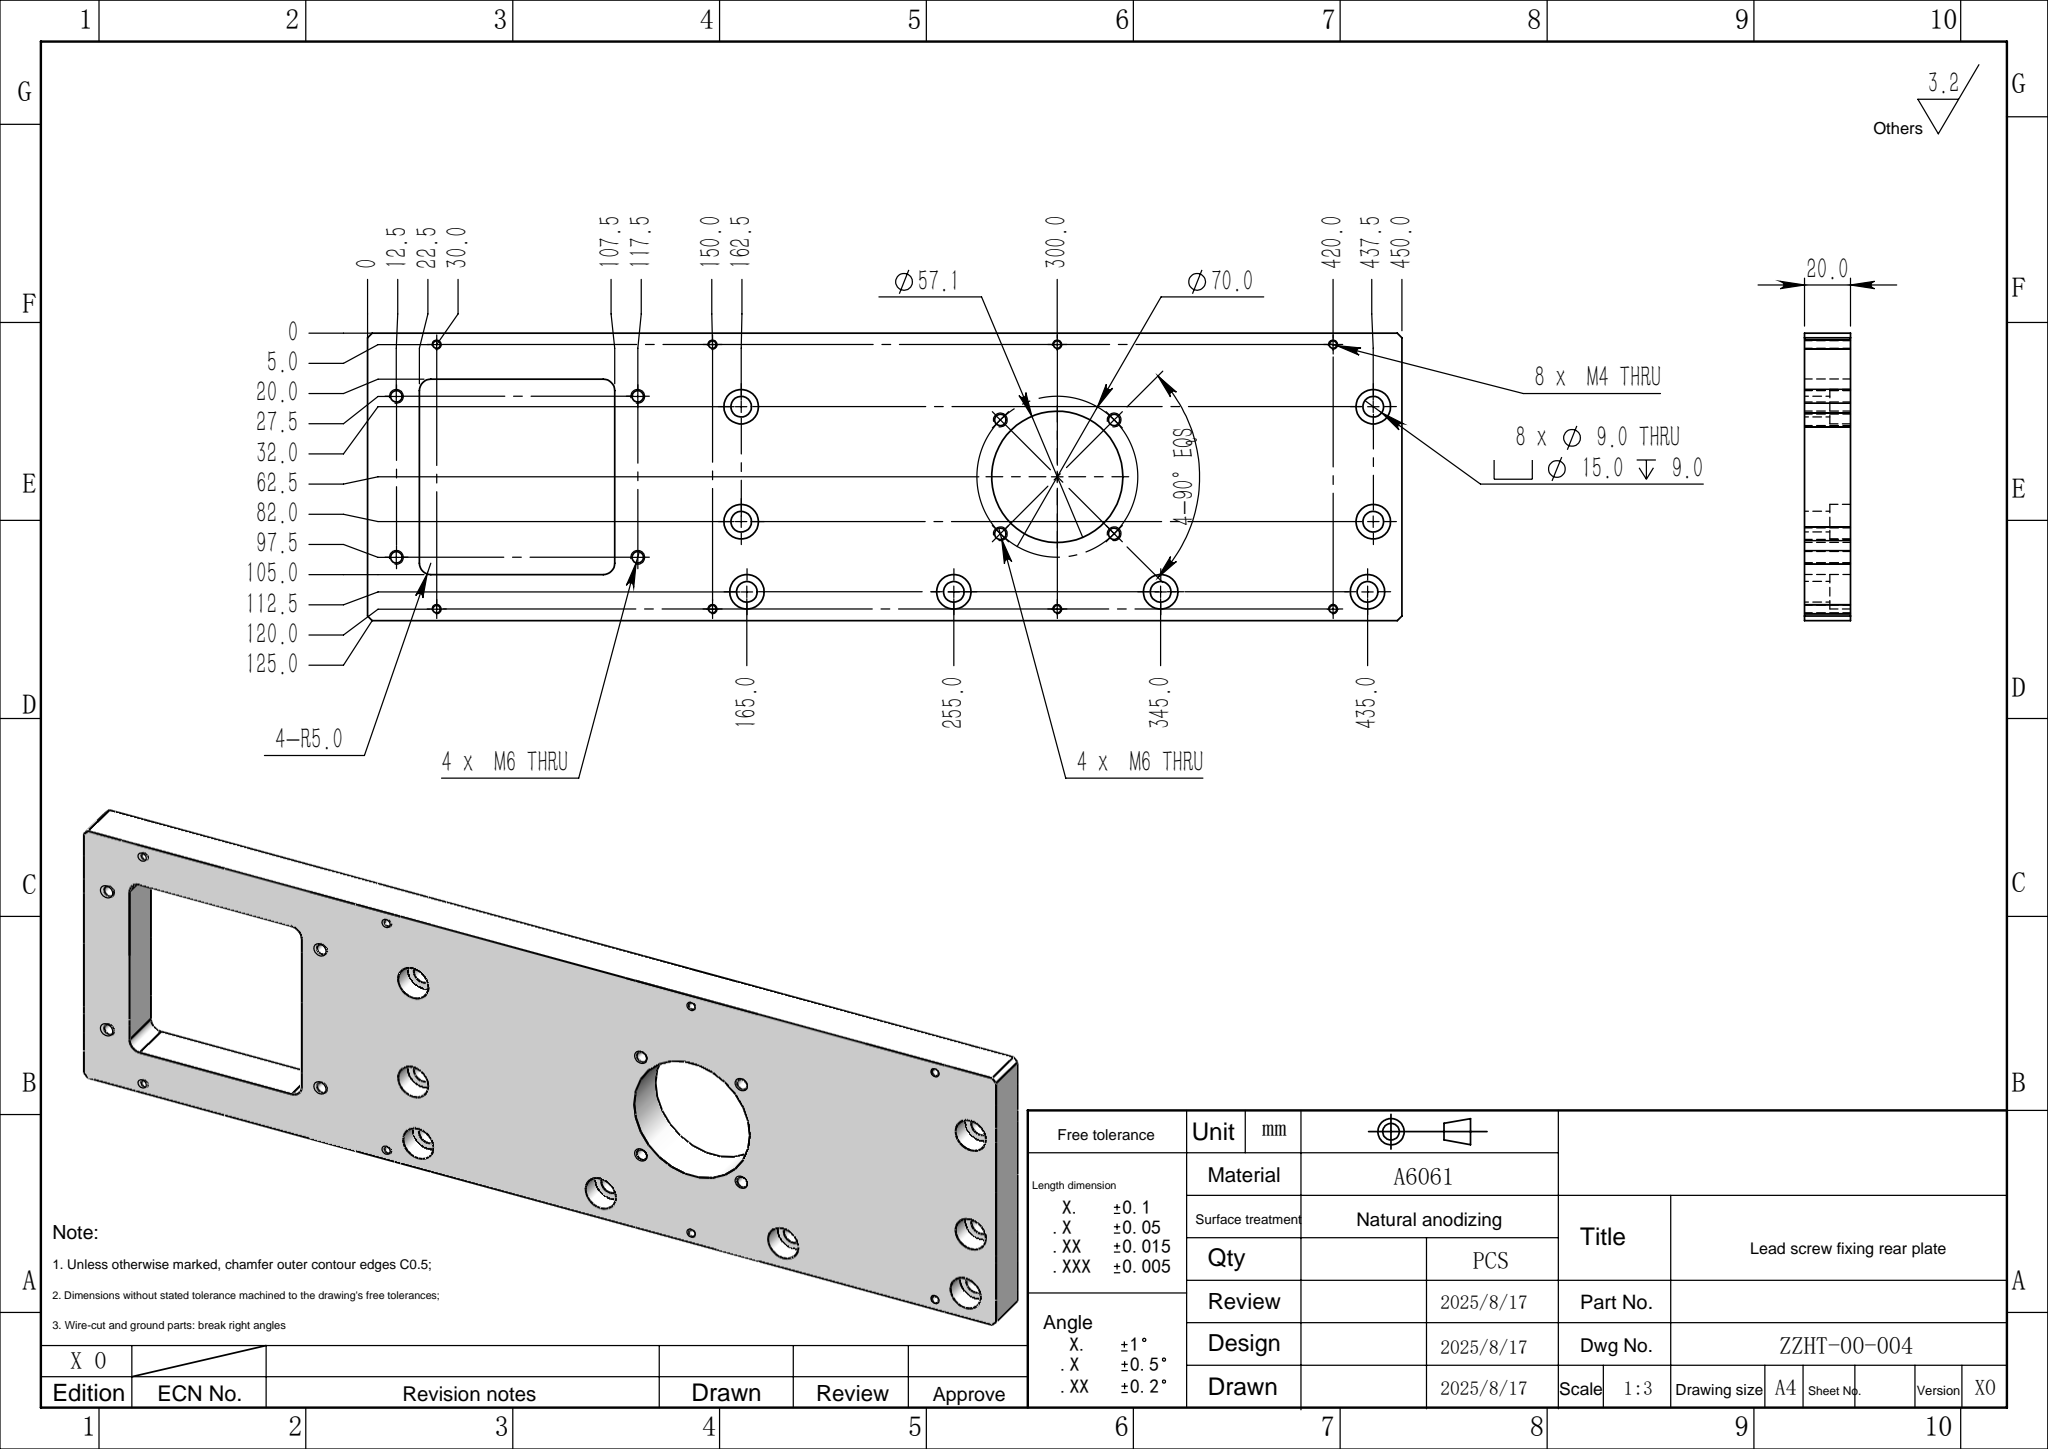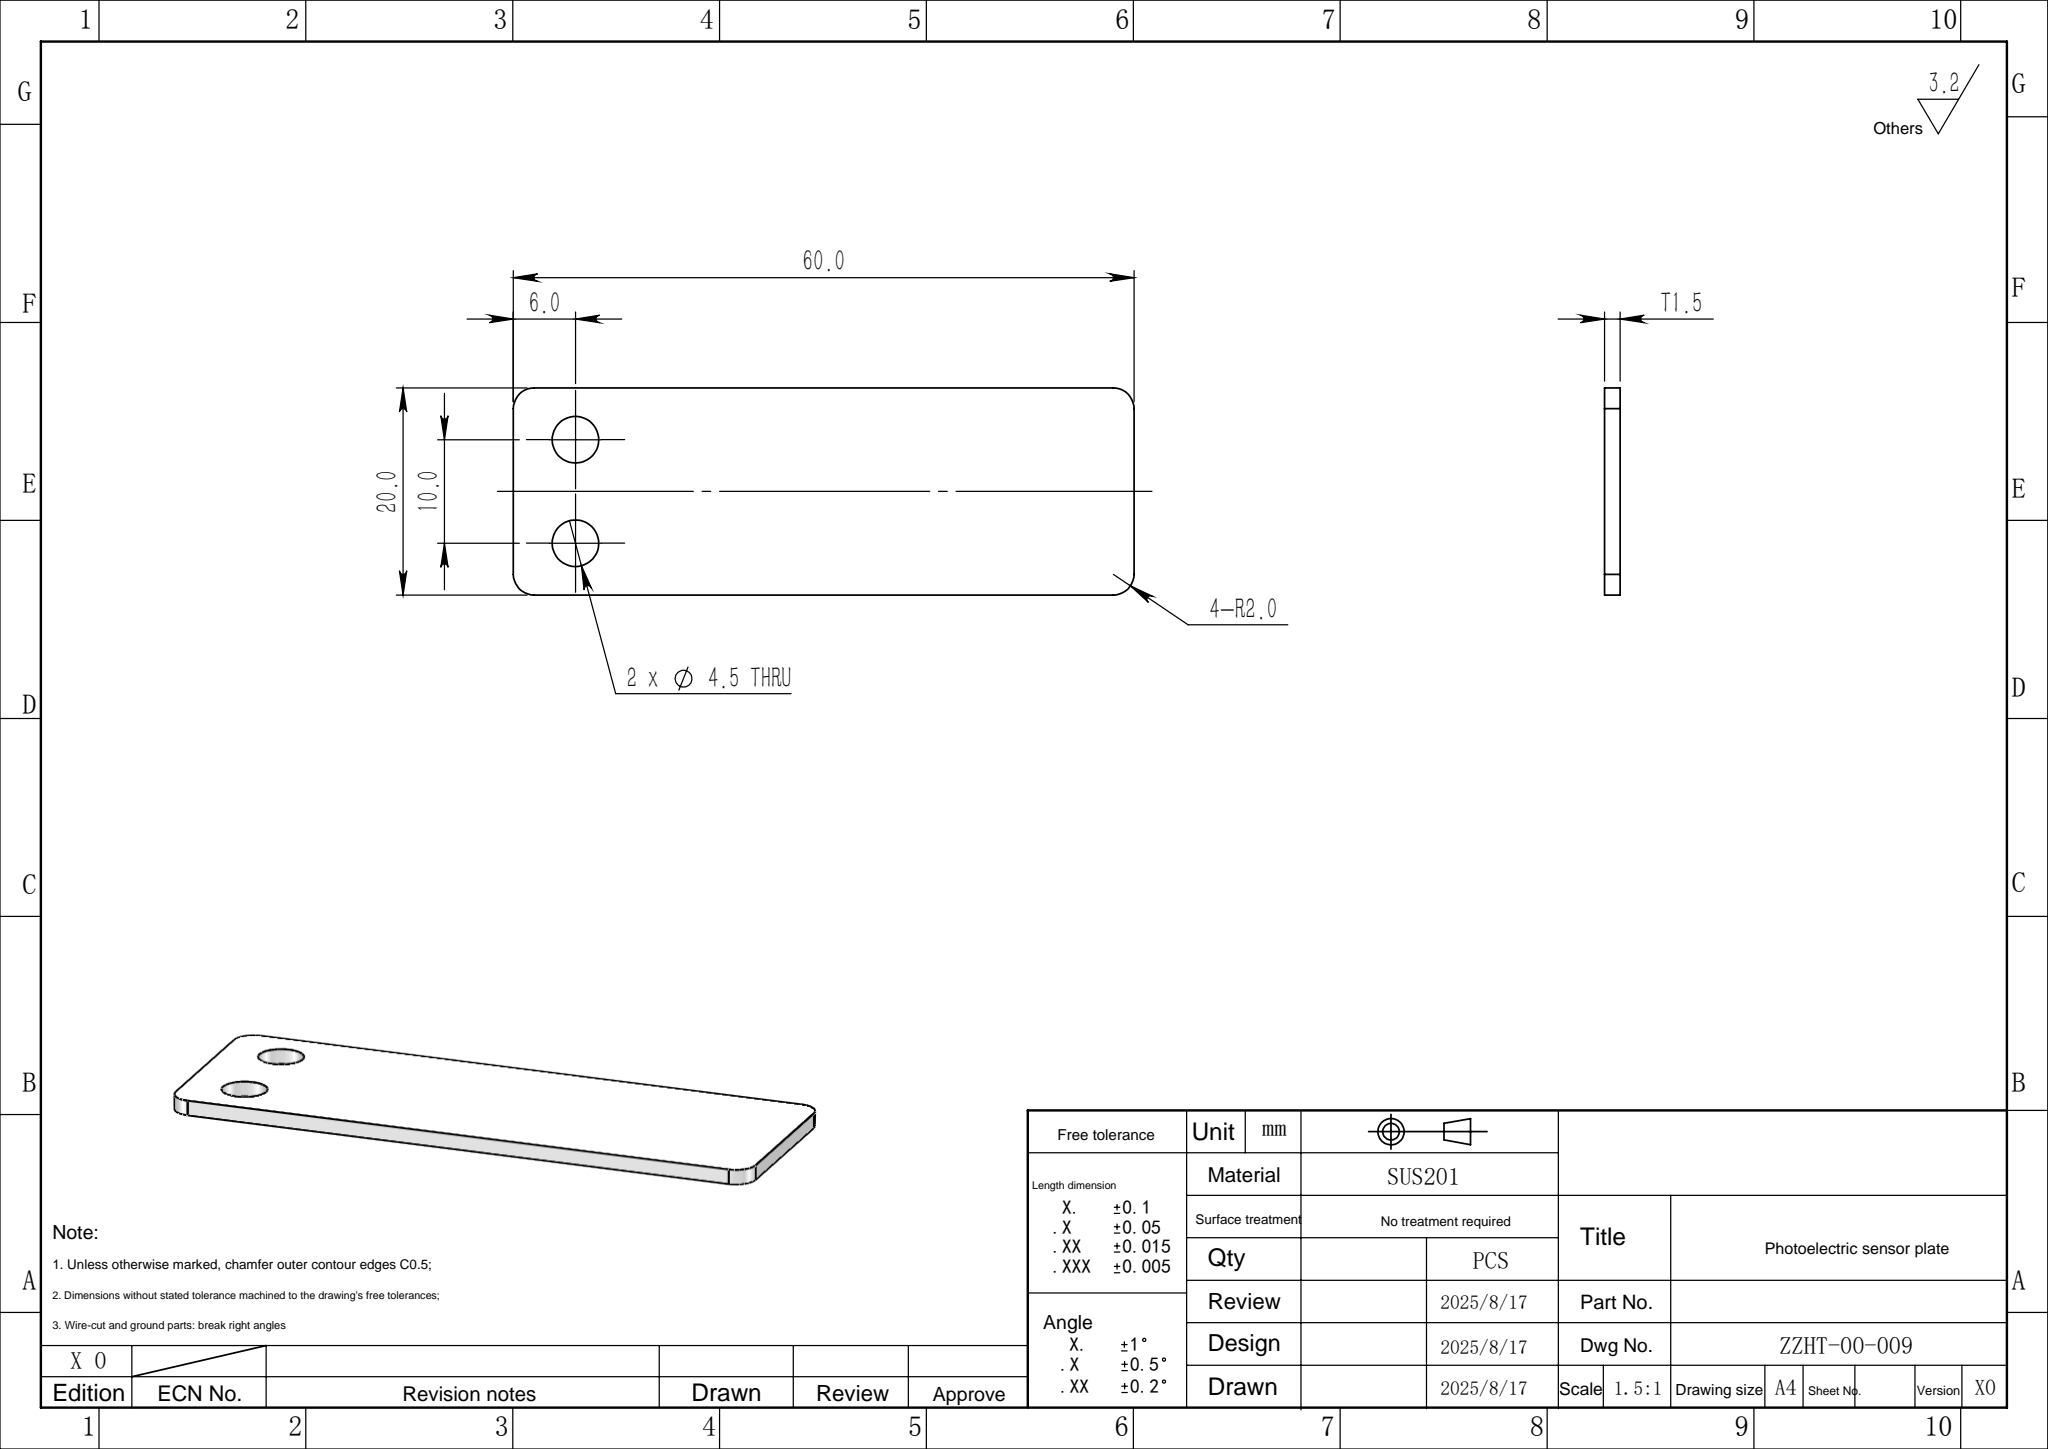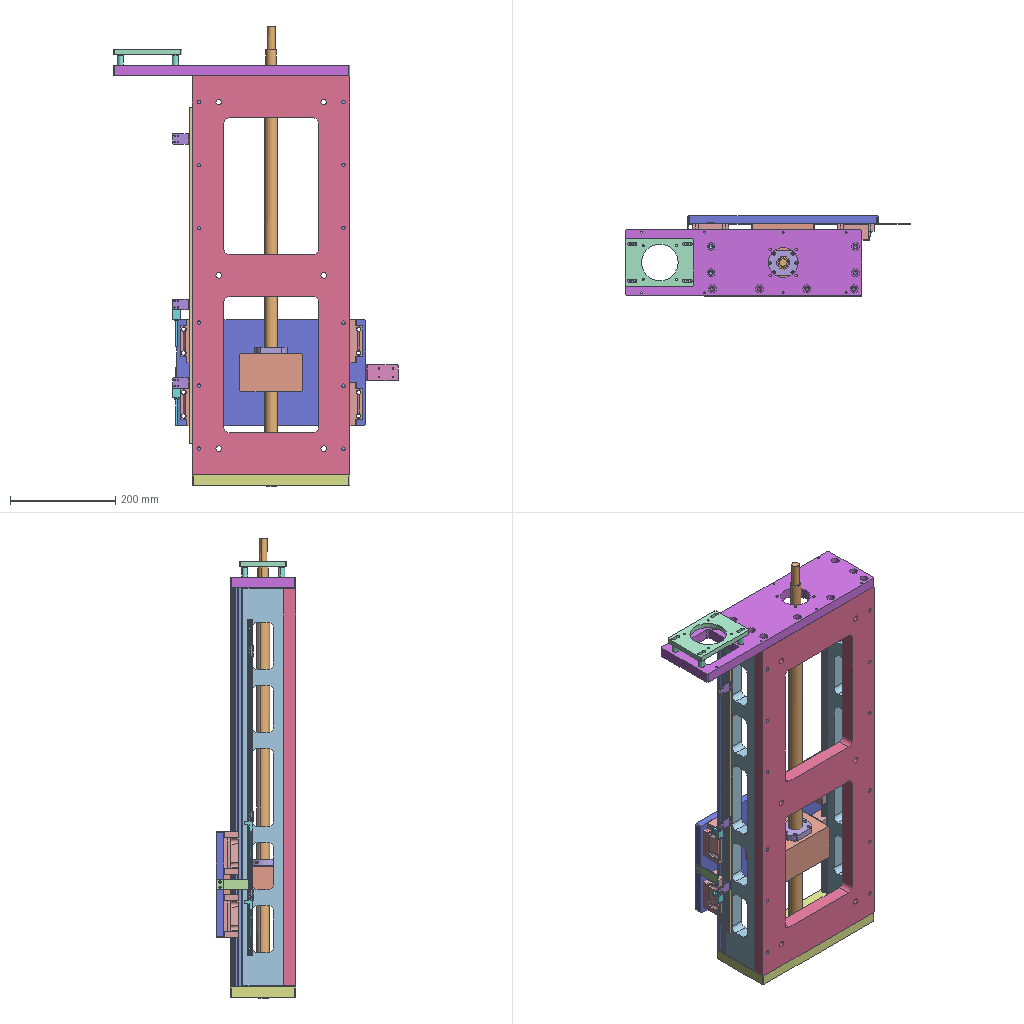Assembly | SolidWorks | 5 different items | 5 placed | box 542 x 152 x 876 mm
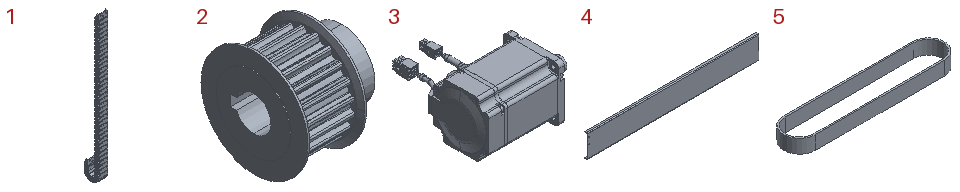Parts list (item | quantity | size | volume | features):
1 | x1 | - | 252756 mm3 | features BaseBody 43
2 | x1 | 48 x 57.9 x 57.9 mm | 58818 mm3 | features BaseBody 1
3 | x1 | 147.2 x 164.554 x 80 mm | 672337 mm3 | features BaseBody 7
4 | x1 | 740 x 12 x 100 mm | 174224 mm3 | features HoleWzd 2, EdgeFlange 1, Fillet 1, FlatPattern 1, SMBaseFlange 1, SheetMetal 1
5 | x1 | 293.56 x 58.56 x 25 mm | 48341 mm3 | features BeltProfileFeature 1, ExtruThin 1
Mates (type | each side: item.copy, entity, surface, feature):
Concentric | 3.1 face | 2.1 face
BeltDim | 2.1 face | assembly face